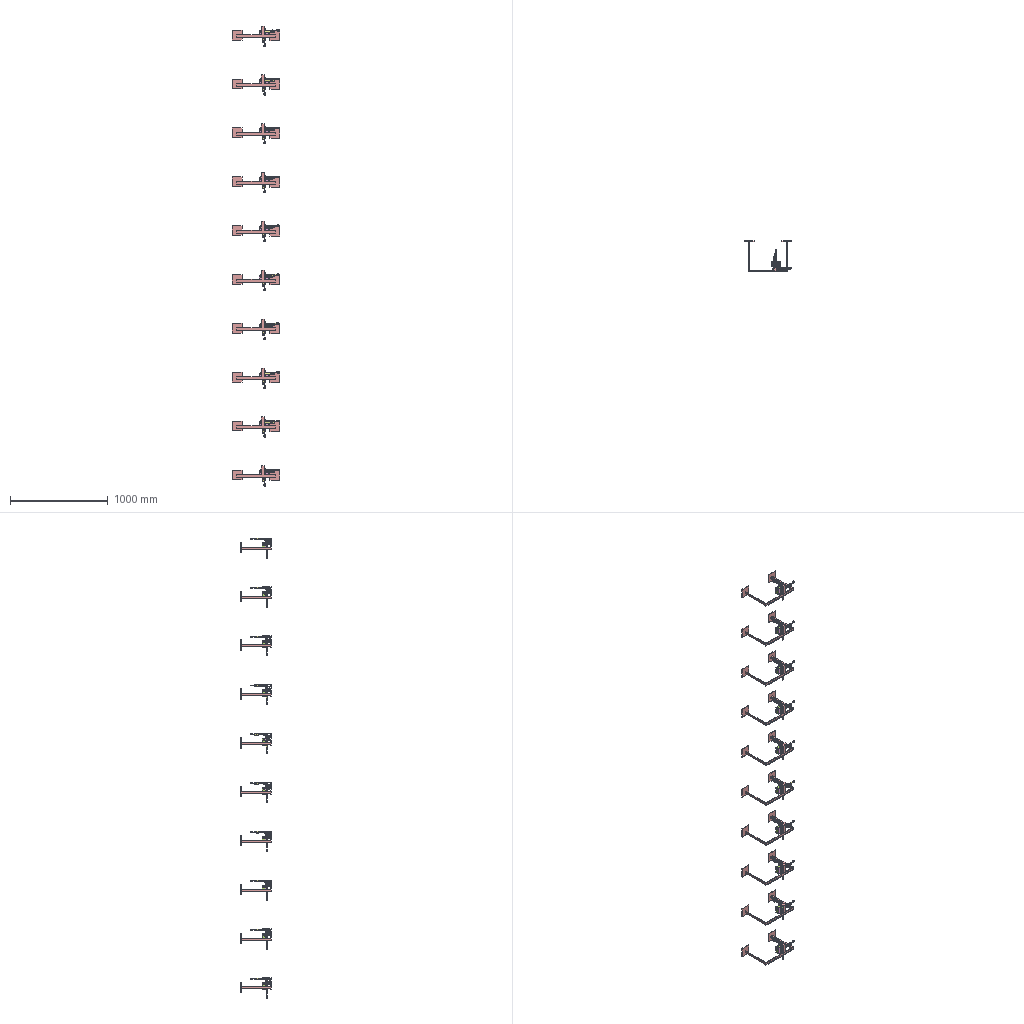Assembly | SolidWorks | 8 different items | 120 placed | box 486 x 308 x 4707 mm
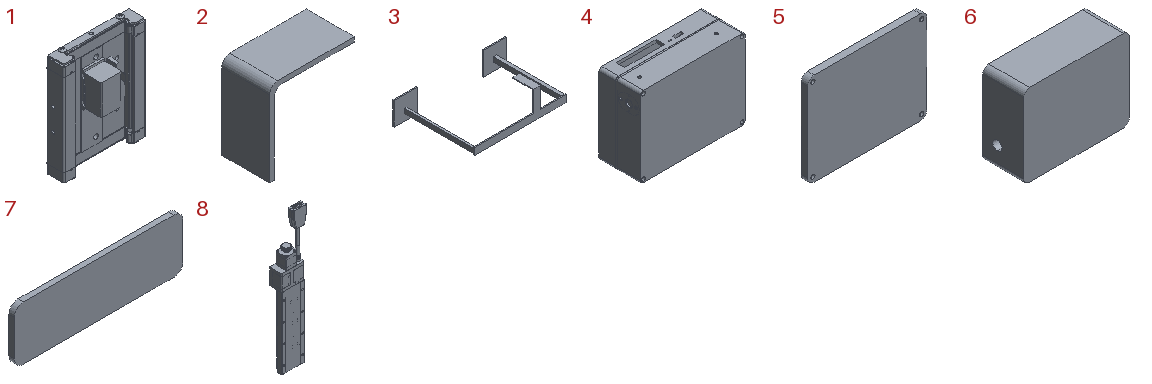Parts list (item | quantity | size | volume | features):
1 | x30 | 30 x 10.5 x 39.416 mm | 4914 mm3 | features BaseBody 23, Scale 1
2 | x10 | 53 x 30 x 53 mm | 9270 mm3 | features Extrusion 1
3 | x10 | 485.708 x 308 x 149.774 mm | 313754 mm3 | features ICE 5, BaseBody 1, MoveFace 1
4 | x10 | 77 x 28.5 x 55 mm | 24995 mm3 | features BaseBody 1
5 | x10 | 90 x 5 x 70 mm | 30997 mm3 | features Extrusion 1, ICE 1
6 | x10 | 90 x 35 x 70 mm | 61634 mm3 | features ICE 2, Extrusion 1, Fillet 1, HoleWzd 1
7 | x10 | 94 x 3 x 30 mm | 8396 mm3 | features Extrusion 1, Fillet 1
8 | x30 | - | - | features BaseBody 2, RefSurface 1, Scale 1
Mates (type | each side: item.copy, entity, surface, feature):
Coincident | 4.1 face plane Input 1 | 6.1 face plane Cut-Extrude1
Parallel | 4.1 face plane Input 1 | 6.1 face plane Cut-Extrude1
DistanceDim | 6.1 face plane Cut-Extrude1 | 4.1 face plane Input 1 | 2 times
Coincident | 6.1 face plane Boss-Extrude1 | 5.1 face plane Boss-Extrude1
Concentric | 6.1 face cylinder M3 Tapped Hole1 | 5.1 face cylinder Cut-Extrude1 | 2 times
Coincident | 5.1 face plane Boss-Extrude1 | 7.1 face plane Boss-Extrude1 | 2 times
Coincident | 8.1 face plane Surface-Input 1 | 7.1 face plane Boss-Extrude1 | 3 times
DistanceDim | 7.1 face plane Boss-Extrude1 | 6.1 face plane Boss-Extrude1
Concentric | 8.1 face cylinder Surface-Input 1 | 1.1 face cylinder Input 24
Parallel | 5.1 face plane Boss-Extrude1 | 1.1 face plane Input 2
Coincident | 1.1 face plane Input 2 | 8.2 face plane Surface-Input 1
Concentric | 8.2 face cylinder Surface-Input 1 | 1.2 face cylinder Input 24
Parallel | 8.2 face plane Surface-Input 1 | 1.2 face plane Input 2
Coincident | 3.1 face plane Boss-Extrude1 | 8.3 face plane Surface-Input 1 | 2 times
DistanceDim | 8.3 face plane Surface-Input 1 | 3.1 face plane Input 1
Concentric | 8.3 face cylinder Surface-Input 1 | 1.3 face cylinder Input 24
Parallel | 3.1 face plane Boss-Extrude1 | 1.3 face plane Input 2
Concentric | 1.1 edge | 8.2 face cylinder Surface-Input 1
Concentric | 1.1 face cylinder Input 2 | 8.2 face cylinder Surface-Input 1
Coincident | 1.3 face plane Input 2 | 2.1 face plane Boss-Extrude1 | 3 times
Coincident | 1.2 face plane Input 2 | 2.1 face plane Boss-Extrude1 | 3 times